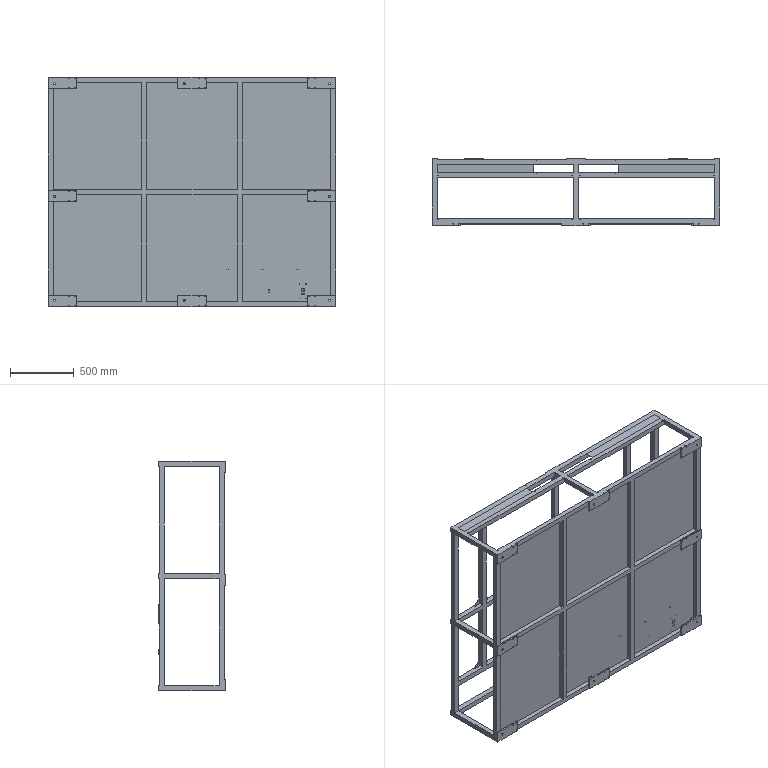Part | STEP file | 1 solid | 530 faces | box 2260 x 525 x 1800 mm | volume 63757591 mm3 | plane 274 | cylinder 190 | cone 66 | commonest cylinder face diameters 6.8 x90 7 x32 3.3 x24 5 x16 14 x16 8 x12